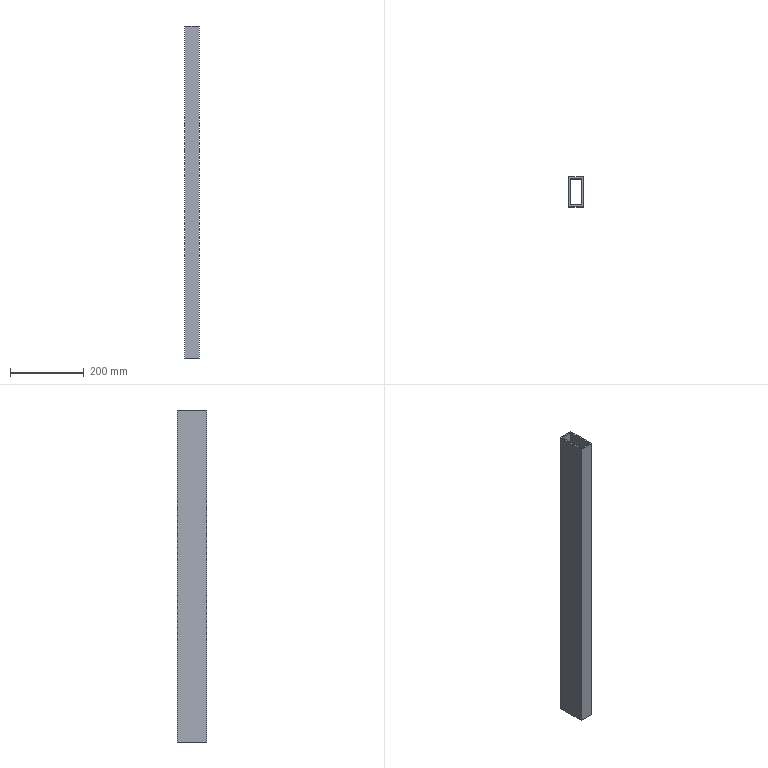Part | SolidWorks | features Extrusion 1 | 1 solid | 10 faces | box 40 x 80 x 900 mm | volume 806400 mm3 | plane 10
STEP:
#1=CARTESIAN_POINT('',(-20.,40.,450.));
#2=VERTEX_POINT('',#1);
#3=CARTESIAN_POINT('',(-20.,-40.,450.));
#4=VERTEX_POINT('',#3);
#5=CARTESIAN_POINT('',(-20.,40.,450.));
#6=DIRECTION('',(0.,-1.,0.));
#7=VECTOR('',#6,1000.);
#8=LINE('',#5,#7);
#9=EDGE_CURVE('',#2,#4,#8,.T.);
#10=ORIENTED_EDGE('',*,*,#9,.F.);
#11=CARTESIAN_POINT('',(-20.,40.,-450.));
#12=VERTEX_POINT('',#11);
#13=CARTESIAN_POINT('',(-20.,40.,-450.));
#14=DIRECTION('',(0.,0.,1.));
#15=VECTOR('',#14,1000.);
#16=LINE('',#13,#15);
#17=EDGE_CURVE('',#12,#2,#16,.T.);
#18=ORIENTED_EDGE('',*,*,#17,.F.);
#19=CARTESIAN_POINT('',(-20.,-40.,-450.));
#20=VERTEX_POINT('',#19);
#21=CARTESIAN_POINT('',(-20.,40.,-450.));
#22=DIRECTION('',(0.,-1.,0.));
#23=VECTOR('',#22,1000.);
#24=LINE('',#21,#23);
#25=EDGE_CURVE('',#12,#20,#24,.T.);
#26=ORIENTED_EDGE('',*,*,#25,.T.);
#27=CARTESIAN_POINT('',(-20.,-40.,-450.));
#28=DIRECTION('',(0.,0.,1.));
#29=VECTOR('',#28,1000.);
#30=LINE('',#27,#29);
#31=EDGE_CURVE('',#20,#4,#30,.T.);
#32=ORIENTED_EDGE('',*,*,#31,.T.);
#33=EDGE_LOOP('',(#10,#18,#26,#32));
#34=FACE_OUTER_BOUND('',#33,.T.);
#35=CARTESIAN_POINT('',(-20.,40.,-450.));
#36=DIRECTION('',(-1.,0.,0.));
#37=DIRECTION('',(0.,0.,1.));
#38=AXIS2_PLACEMENT_3D('',#35,#36,#37);
#39=PLANE('',#38);
#40=ADVANCED_FACE('',(#34),#39,.T.);
#41=CARTESIAN_POINT('',(20.,40.,450.));
#42=VERTEX_POINT('',#41);
#43=CARTESIAN_POINT('',(20.,40.,450.));
#44=DIRECTION('',(-1.,0.,0.));
#45=VECTOR('',#44,1000.);
#46=LINE('',#43,#45);
#47=EDGE_CURVE('',#42,#2,#46,.T.);
#48=ORIENTED_EDGE('',*,*,#47,.F.);
#49=CARTESIAN_POINT('',(20.,40.,-450.));
#50=VERTEX_POINT('',#49);
#51=CARTESIAN_POINT('',(20.,40.,-450.));
#52=DIRECTION('',(0.,0.,1.));
#53=VECTOR('',#52,1000.);
#54=LINE('',#51,#53);
#55=EDGE_CURVE('',#50,#42,#54,.T.);
#56=ORIENTED_EDGE('',*,*,#55,.F.);
#57=CARTESIAN_POINT('',(20.,40.,-450.));
#58=DIRECTION('',(-1.,0.,0.));
#59=VECTOR('',#58,1000.);
#60=LINE('',#57,#59);
#61=EDGE_CURVE('',#50,#12,#60,.T.);
#62=ORIENTED_EDGE('',*,*,#61,.T.);
#63=ORIENTED_EDGE('',*,*,#17,.T.);
#64=EDGE_LOOP('',(#48,#56,#62,#63));
#65=FACE_OUTER_BOUND('',#64,.T.);
#66=CARTESIAN_POINT('',(20.,40.,-450.));
#67=DIRECTION('',(0.,1.,0.));
#68=DIRECTION('',(0.,0.,1.));
#69=AXIS2_PLACEMENT_3D('',#66,#67,#68);
#70=PLANE('',#69);
#71=ADVANCED_FACE('',(#65),#70,.T.);
#72=CARTESIAN_POINT('',(20.,-40.,450.));
#73=VERTEX_POINT('',#72);
#74=CARTESIAN_POINT('',(20.,-40.,450.));
#75=DIRECTION('',(0.,1.,0.));
#76=VECTOR('',#75,1000.);
#77=LINE('',#74,#76);
#78=EDGE_CURVE('',#73,#42,#77,.T.);
#79=ORIENTED_EDGE('',*,*,#78,.F.);
#80=CARTESIAN_POINT('',(20.,-40.,-450.));
#81=VERTEX_POINT('',#80);
#82=CARTESIAN_POINT('',(20.,-40.,-450.));
#83=DIRECTION('',(0.,0.,1.));
#84=VECTOR('',#83,1000.);
#85=LINE('',#82,#84);
#86=EDGE_CURVE('',#81,#73,#85,.T.);
#87=ORIENTED_EDGE('',*,*,#86,.F.);
#88=CARTESIAN_POINT('',(20.,-40.,-450.));
#89=DIRECTION('',(0.,1.,0.));
#90=VECTOR('',#89,1000.);
#91=LINE('',#88,#90);
#92=EDGE_CURVE('',#81,#50,#91,.T.);
#93=ORIENTED_EDGE('',*,*,#92,.T.);
#94=ORIENTED_EDGE('',*,*,#55,.T.);
#95=EDGE_LOOP('',(#79,#87,#93,#94));
#96=FACE_OUTER_BOUND('',#95,.T.);
#97=CARTESIAN_POINT('',(20.,-40.,-450.));
#98=DIRECTION('',(1.,0.,0.));
#99=DIRECTION('',(0.,0.,-1.));
#100=AXIS2_PLACEMENT_3D('',#97,#98,#99);
#101=PLANE('',#100);
#102=ADVANCED_FACE('',(#96),#101,.T.);
#103=CARTESIAN_POINT('',(-20.,-40.,450.));
#104=DIRECTION('',(1.,0.,0.));
#105=VECTOR('',#104,1000.);
#106=LINE('',#103,#105);
#107=EDGE_CURVE('',#4,#73,#106,.T.);
#108=ORIENTED_EDGE('',*,*,#107,.F.);
#109=ORIENTED_EDGE('',*,*,#31,.F.);
#110=CARTESIAN_POINT('',(-20.,-40.,-450.));
#111=DIRECTION('',(1.,0.,0.));
#112=VECTOR('',#111,1000.);
#113=LINE('',#110,#112);
#114=EDGE_CURVE('',#20,#81,#113,.T.);
#115=ORIENTED_EDGE('',*,*,#114,.T.);
#116=ORIENTED_EDGE('',*,*,#86,.T.);
#117=EDGE_LOOP('',(#108,#109,#115,#116));
#118=FACE_OUTER_BOUND('',#117,.T.);
#119=CARTESIAN_POINT('',(-20.,-40.,-450.));
#120=DIRECTION('',(0.,-1.,0.));
#121=DIRECTION('',(0.,0.,-1.));
#122=AXIS2_PLACEMENT_3D('',#119,#120,#121);
#123=PLANE('',#122);
#124=ADVANCED_FACE('',(#118),#123,.T.);
#125=CARTESIAN_POINT('',(16.,36.,-450.));
#126=VERTEX_POINT('',#125);
#127=CARTESIAN_POINT('',(-16.,36.,-450.));
#128=VERTEX_POINT('',#127);
#129=CARTESIAN_POINT('',(16.,36.,-450.));
#130=DIRECTION('',(-1.,0.,0.));
#131=VECTOR('',#130,1000.);
#132=LINE('',#129,#131);
#133=EDGE_CURVE('',#126,#128,#132,.T.);
#134=ORIENTED_EDGE('',*,*,#133,.T.);
#135=CARTESIAN_POINT('',(-16.,-36.,-450.));
#136=VERTEX_POINT('',#135);
#137=CARTESIAN_POINT('',(-16.,36.,-450.));
#138=DIRECTION('',(0.,-1.,0.));
#139=VECTOR('',#138,1000.);
#140=LINE('',#137,#139);
#141=EDGE_CURVE('',#128,#136,#140,.T.);
#142=ORIENTED_EDGE('',*,*,#141,.T.);
#143=CARTESIAN_POINT('',(16.,-36.,-450.));
#144=VERTEX_POINT('',#143);
#145=CARTESIAN_POINT('',(-16.,-36.,-450.));
#146=DIRECTION('',(1.,0.,0.));
#147=VECTOR('',#146,1000.);
#148=LINE('',#145,#147);
#149=EDGE_CURVE('',#136,#144,#148,.T.);
#150=ORIENTED_EDGE('',*,*,#149,.T.);
#151=CARTESIAN_POINT('',(16.,-36.,-450.));
#152=DIRECTION('',(0.,1.,0.));
#153=VECTOR('',#152,1000.);
#154=LINE('',#151,#153);
#155=EDGE_CURVE('',#144,#126,#154,.T.);
#156=ORIENTED_EDGE('',*,*,#155,.T.);
#157=EDGE_LOOP('',(#134,#142,#150,#156));
#158=FACE_BOUND('',#157,.T.);
#159=ORIENTED_EDGE('',*,*,#25,.F.);
#160=ORIENTED_EDGE('',*,*,#61,.F.);
#161=ORIENTED_EDGE('',*,*,#92,.F.);
#162=ORIENTED_EDGE('',*,*,#114,.F.);
#163=EDGE_LOOP('',(#159,#160,#161,#162));
#164=FACE_OUTER_BOUND('',#163,.T.);
#165=CARTESIAN_POINT('',(0.,0.,-450.));
#166=DIRECTION('',(0.,0.,1.));
#167=DIRECTION('',(1.,0.,0.));
#168=AXIS2_PLACEMENT_3D('',#165,#166,#167);
#169=PLANE('',#168);
#170=ADVANCED_FACE('',(#158,#164),#169,.F.);
#171=CARTESIAN_POINT('',(-16.,36.,450.));
#172=VERTEX_POINT('',#171);
#173=CARTESIAN_POINT('',(-16.,-36.,450.));
#174=VERTEX_POINT('',#173);
#175=CARTESIAN_POINT('',(-16.,36.,450.));
#176=DIRECTION('',(0.,-1.,0.));
#177=VECTOR('',#176,1000.);
#178=LINE('',#175,#177);
#179=EDGE_CURVE('',#172,#174,#178,.T.);
#180=ORIENTED_EDGE('',*,*,#179,.F.);
#181=CARTESIAN_POINT('',(16.,36.,450.));
#182=VERTEX_POINT('',#181);
#183=CARTESIAN_POINT('',(16.,36.,450.));
#184=DIRECTION('',(-1.,0.,0.));
#185=VECTOR('',#184,1000.);
#186=LINE('',#183,#185);
#187=EDGE_CURVE('',#182,#172,#186,.T.);
#188=ORIENTED_EDGE('',*,*,#187,.F.);
#189=CARTESIAN_POINT('',(16.,-36.,450.));
#190=VERTEX_POINT('',#189);
#191=CARTESIAN_POINT('',(16.,-36.,450.));
#192=DIRECTION('',(0.,1.,0.));
#193=VECTOR('',#192,1000.);
#194=LINE('',#191,#193);
#195=EDGE_CURVE('',#190,#182,#194,.T.);
#196=ORIENTED_EDGE('',*,*,#195,.F.);
#197=CARTESIAN_POINT('',(-16.,-36.,450.));
#198=DIRECTION('',(1.,0.,0.));
#199=VECTOR('',#198,1000.);
#200=LINE('',#197,#199);
#201=EDGE_CURVE('',#174,#190,#200,.T.);
#202=ORIENTED_EDGE('',*,*,#201,.F.);
#203=EDGE_LOOP('',(#180,#188,#196,#202));
#204=FACE_BOUND('',#203,.T.);
#205=ORIENTED_EDGE('',*,*,#9,.T.);
#206=ORIENTED_EDGE('',*,*,#107,.T.);
#207=ORIENTED_EDGE('',*,*,#78,.T.);
#208=ORIENTED_EDGE('',*,*,#47,.T.);
#209=EDGE_LOOP('',(#205,#206,#207,#208));
#210=FACE_OUTER_BOUND('',#209,.T.);
#211=CARTESIAN_POINT('',(0.,0.,450.));
#212=DIRECTION('',(0.,0.,1.));
#213=DIRECTION('',(1.,0.,0.));
#214=AXIS2_PLACEMENT_3D('',#211,#212,#213);
#215=PLANE('',#214);
#216=ADVANCED_FACE('',(#204,#210),#215,.T.);
#217=ORIENTED_EDGE('',*,*,#179,.T.);
#218=CARTESIAN_POINT('',(-16.,-36.,-450.));
#219=DIRECTION('',(0.,0.,1.));
#220=VECTOR('',#219,1000.);
#221=LINE('',#218,#220);
#222=EDGE_CURVE('',#136,#174,#221,.T.);
#223=ORIENTED_EDGE('',*,*,#222,.F.);
#224=ORIENTED_EDGE('',*,*,#141,.F.);
#225=CARTESIAN_POINT('',(-16.,36.,-450.));
#226=DIRECTION('',(0.,0.,1.));
#227=VECTOR('',#226,1000.);
#228=LINE('',#225,#227);
#229=EDGE_CURVE('',#128,#172,#228,.T.);
#230=ORIENTED_EDGE('',*,*,#229,.T.);
#231=EDGE_LOOP('',(#217,#223,#224,#230));
#232=FACE_OUTER_BOUND('',#231,.T.);
#233=CARTESIAN_POINT('',(-16.,36.,-450.));
#234=DIRECTION('',(-1.,0.,0.));
#235=DIRECTION('',(0.,0.,1.));
#236=AXIS2_PLACEMENT_3D('',#233,#234,#235);
#237=PLANE('',#236);
#238=ADVANCED_FACE('',(#232),#237,.F.);
#239=ORIENTED_EDGE('',*,*,#187,.T.);
#240=ORIENTED_EDGE('',*,*,#229,.F.);
#241=ORIENTED_EDGE('',*,*,#133,.F.);
#242=CARTESIAN_POINT('',(16.,36.,-450.));
#243=DIRECTION('',(0.,0.,1.));
#244=VECTOR('',#243,1000.);
#245=LINE('',#242,#244);
#246=EDGE_CURVE('',#126,#182,#245,.T.);
#247=ORIENTED_EDGE('',*,*,#246,.T.);
#248=EDGE_LOOP('',(#239,#240,#241,#247));
#249=FACE_OUTER_BOUND('',#248,.T.);
#250=CARTESIAN_POINT('',(16.,36.,-450.));
#251=DIRECTION('',(0.,1.,0.));
#252=DIRECTION('',(0.,0.,1.));
#253=AXIS2_PLACEMENT_3D('',#250,#251,#252);
#254=PLANE('',#253);
#255=ADVANCED_FACE('',(#249),#254,.F.);
#256=ORIENTED_EDGE('',*,*,#195,.T.);
#257=ORIENTED_EDGE('',*,*,#246,.F.);
#258=ORIENTED_EDGE('',*,*,#155,.F.);
#259=CARTESIAN_POINT('',(16.,-36.,-450.));
#260=DIRECTION('',(0.,0.,1.));
#261=VECTOR('',#260,1000.);
#262=LINE('',#259,#261);
#263=EDGE_CURVE('',#144,#190,#262,.T.);
#264=ORIENTED_EDGE('',*,*,#263,.T.);
#265=EDGE_LOOP('',(#256,#257,#258,#264));
#266=FACE_OUTER_BOUND('',#265,.T.);
#267=CARTESIAN_POINT('',(16.,-36.,-450.));
#268=DIRECTION('',(1.,0.,0.));
#269=DIRECTION('',(0.,0.,-1.));
#270=AXIS2_PLACEMENT_3D('',#267,#268,#269);
#271=PLANE('',#270);
#272=ADVANCED_FACE('',(#266),#271,.F.);
#273=ORIENTED_EDGE('',*,*,#201,.T.);
#274=ORIENTED_EDGE('',*,*,#263,.F.);
#275=ORIENTED_EDGE('',*,*,#149,.F.);
#276=ORIENTED_EDGE('',*,*,#222,.T.);
#277=EDGE_LOOP('',(#273,#274,#275,#276));
#278=FACE_OUTER_BOUND('',#277,.T.);
#279=CARTESIAN_POINT('',(-16.,-36.,-450.));
#280=DIRECTION('',(0.,-1.,0.));
#281=DIRECTION('',(0.,0.,-1.));
#282=AXIS2_PLACEMENT_3D('',#279,#280,#281);
#283=PLANE('',#282);
#284=ADVANCED_FACE('',(#278),#283,.F.);
#285=CLOSED_SHELL('',(#40,#71,#102,#124,#170,#216,#238,#255,#272,#284));
#286=MANIFOLD_SOLID_BREP('',#285);
#287=CARTESIAN_POINT('',(0.,0.,0.));
#288=DIRECTION('',(0.,0.,1.));
#289=DIRECTION('',(1.,0.,0.));
#290=AXIS2_PLACEMENT_3D('',#287,#288,#289);
#291=(LENGTH_UNIT()NAMED_UNIT(*)SI_UNIT(.MILLI.,.METRE.));
#292=UNCERTAINTY_MEASURE_WITH_UNIT(LENGTH_MEASURE(0.00001),#291,'','');
#293=(NAMED_UNIT(*)PLANE_ANGLE_UNIT()SI_UNIT($,.RADIAN.));
#294=(NAMED_UNIT(*)SI_UNIT($,.STERADIAN.)SOLID_ANGLE_UNIT());
#295=(GEOMETRIC_REPRESENTATION_CONTEXT(3)GLOBAL_UNCERTAINTY_ASSIGNED_CONTEXT((#292))GLOBAL_UNIT_ASSIGNED_CONTEXT((#291,#293,#294))REPRESENTATION_CONTEXT('',''));
#296=ADVANCED_BREP_SHAPE_REPRESENTATION('',(#286,#290),#295);